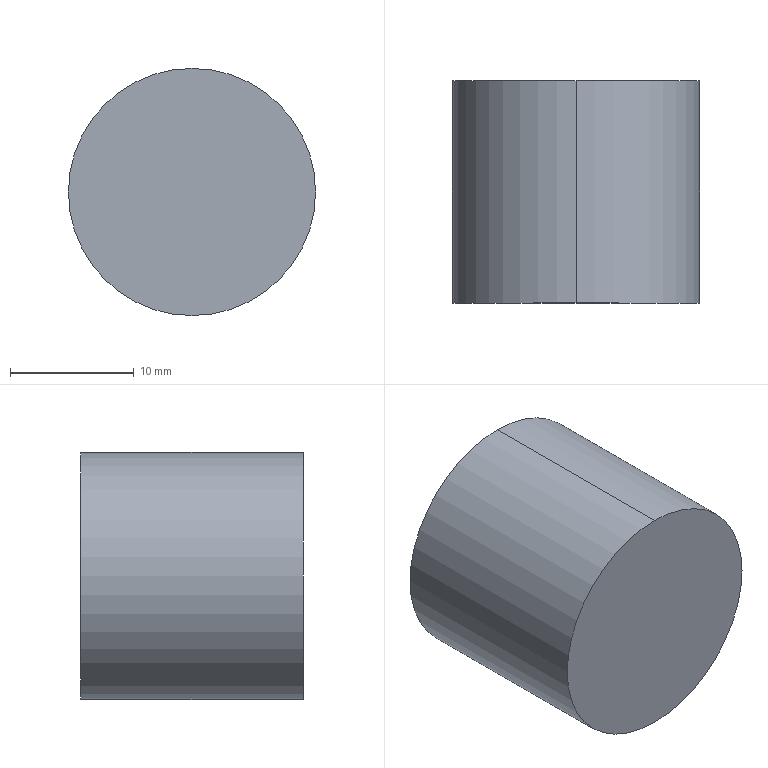Part | STEP file | OP10-158_seal pad (valve guide) | 1 solid | 11 faces | box 20 x 18 x 20 mm | volume 4188 mm3 | cylinder 6 | plane 3 | cone 2 | commonest cylinder face diameters 10 x2 14 x2 20 x2
STEP:
#1=CARTESIAN_POINT('',(0.,0.,0.));
#2=DIRECTION('',(0.,0.,1.));
#3=DIRECTION('',(1.,0.,0.));
#4=AXIS2_PLACEMENT_3D('',#1,#2,#3);
#5=CARTESIAN_POINT('',(0.,7.,5.));
#6=VERTEX_POINT('',#5);
#7=CARTESIAN_POINT('',(0.,11.,5.));
#8=VERTEX_POINT('',#7);
#9=CARTESIAN_POINT('',(0.,18.,5.));
#10=DIRECTION('',(0.,1.,0.));
#11=VECTOR('',#10,1.);
#12=LINE('',#9,#11);
#13=CARTESIAN_POINT('',(0.,18.,0.));
#14=DIRECTION('',(0.,1.,0.));
#15=DIRECTION('',(0.,0.,1.));
#16=AXIS2_PLACEMENT_3D('',#13,#14,#15);
#17=CYLINDRICAL_SURFACE('',#16,5.);
#18=CARTESIAN_POINT('',(6.283,0.));
#19=DIRECTION('',(0.,1.));
#20=VECTOR('',#19,1.);
#21=LINE('',#18,#20);
#22=(GEOMETRIC_REPRESENTATION_CONTEXT(2)PARAMETRIC_REPRESENTATION_CONTEXT()REPRESENTATION_CONTEXT('',''));
#23=DEFINITIONAL_REPRESENTATION('',(#21),#22);
#24=PCURVE('',#17,#23);
#25=CARTESIAN_POINT('',(0.,18.,0.));
#26=DIRECTION('',(0.,1.,0.));
#27=DIRECTION('',(0.,0.,1.));
#28=AXIS2_PLACEMENT_3D('',#25,#26,#27);
#29=CYLINDRICAL_SURFACE('',#28,5.);
#30=CARTESIAN_POINT('',(0.,0.));
#31=DIRECTION('',(0.,1.));
#32=VECTOR('',#31,1.);
#33=LINE('',#30,#32);
#34=(GEOMETRIC_REPRESENTATION_CONTEXT(2)PARAMETRIC_REPRESENTATION_CONTEXT()REPRESENTATION_CONTEXT('',''));
#35=DEFINITIONAL_REPRESENTATION('',(#33),#34);
#36=PCURVE('',#29,#35);
#37=SURFACE_CURVE('',#12,(#24,#36),.PCURVE_S1.);
#38=EDGE_CURVE('',#6,#8,#37,.T.);
#39=ORIENTED_EDGE('',*,*,#38,.T.);
#40=CARTESIAN_POINT('',(0.,11.,-5.));
#41=VERTEX_POINT('',#40);
#42=CARTESIAN_POINT('',(0.,11.,0.));
#43=DIRECTION('',(0.,-1.,0.));
#44=DIRECTION('',(0.,0.,1.));
#45=AXIS2_PLACEMENT_3D('',#42,#43,#44);
#46=CIRCLE('',#45,5.);
#47=CARTESIAN_POINT('',(6.283,-7.));
#48=DIRECTION('',(-1.,0.));
#49=VECTOR('',#48,1.);
#50=LINE('',#47,#49);
#51=(GEOMETRIC_REPRESENTATION_CONTEXT(2)PARAMETRIC_REPRESENTATION_CONTEXT()REPRESENTATION_CONTEXT('',''));
#52=DEFINITIONAL_REPRESENTATION('',(#50),#51);
#53=PCURVE('',#17,#52);
#54=CARTESIAN_POINT('',(0.,11.,0.));
#55=DIRECTION('',(0.,1.,0.));
#56=DIRECTION('',(0.,0.,1.));
#57=AXIS2_PLACEMENT_3D('',#54,#55,#56);
#58=PLANE('',#57);
#59=CARTESIAN_POINT('',(5.,0.));
#60=CARTESIAN_POINT('',(5.,-8.66));
#61=CARTESIAN_POINT('',(-2.5,-4.33));
#62=CARTESIAN_POINT('',(-10.,0.));
#63=CARTESIAN_POINT('',(-2.5,4.33));
#64=CARTESIAN_POINT('',(5.,8.66));
#65=CARTESIAN_POINT('',(5.,0.));
#66=(BOUNDED_CURVE()B_SPLINE_CURVE(2,(#59,#60,#61,#62,#63,#64,#65),.UNSPECIFIED.,.T.,.F.)B_SPLINE_CURVE_WITH_KNOTS((1,2,2,2,2,1),(-2.094,0.,2.094,4.189,6.283,8.378),.UNSPECIFIED.)CURVE()GEOMETRIC_REPRESENTATION_ITEM()RATIONAL_B_SPLINE_CURVE((1.,0.5,1.,0.5,1.,0.5,1.))REPRESENTATION_ITEM(''));
#67=(GEOMETRIC_REPRESENTATION_CONTEXT(2)PARAMETRIC_REPRESENTATION_CONTEXT()REPRESENTATION_CONTEXT('',''));
#68=DEFINITIONAL_REPRESENTATION('',(#66),#67);
#69=PCURVE('',#58,#68);
#70=SURFACE_CURVE('',#46,(#53,#69),.PCURVE_S1.);
#71=EDGE_CURVE('',#8,#41,#70,.T.);
#72=ORIENTED_EDGE('',*,*,#71,.T.);
#73=CARTESIAN_POINT('',(0.,7.,-5.));
#74=VERTEX_POINT('',#73);
#75=CARTESIAN_POINT('',(0.,18.,-5.));
#76=DIRECTION('',(0.,1.,0.));
#77=VECTOR('',#76,1.);
#78=LINE('',#75,#77);
#79=CARTESIAN_POINT('',(3.142,0.));
#80=DIRECTION('',(0.,1.));
#81=VECTOR('',#80,1.);
#82=LINE('',#79,#81);
#83=(GEOMETRIC_REPRESENTATION_CONTEXT(2)PARAMETRIC_REPRESENTATION_CONTEXT()REPRESENTATION_CONTEXT('',''));
#84=DEFINITIONAL_REPRESENTATION('',(#82),#83);
#85=PCURVE('',#17,#84);
#86=CARTESIAN_POINT('',(3.142,0.));
#87=DIRECTION('',(0.,1.));
#88=VECTOR('',#87,1.);
#89=LINE('',#86,#88);
#90=(GEOMETRIC_REPRESENTATION_CONTEXT(2)PARAMETRIC_REPRESENTATION_CONTEXT()REPRESENTATION_CONTEXT('',''));
#91=DEFINITIONAL_REPRESENTATION('',(#89),#90);
#92=PCURVE('',#29,#91);
#93=SURFACE_CURVE('',#78,(#85,#92),.PCURVE_S1.);
#94=EDGE_CURVE('',#74,#41,#93,.T.);
#95=ORIENTED_EDGE('',*,*,#94,.F.);
#96=CARTESIAN_POINT('',(0.,7.,0.));
#97=DIRECTION('',(0.,1.,0.));
#98=DIRECTION('',(0.,0.,1.));
#99=AXIS2_PLACEMENT_3D('',#96,#97,#98);
#100=CIRCLE('',#99,5.);
#101=CARTESIAN_POINT('',(0.,-11.));
#102=DIRECTION('',(1.,0.));
#103=VECTOR('',#102,1.);
#104=LINE('',#101,#103);
#105=(GEOMETRIC_REPRESENTATION_CONTEXT(2)PARAMETRIC_REPRESENTATION_CONTEXT()REPRESENTATION_CONTEXT('',''));
#106=DEFINITIONAL_REPRESENTATION('',(#104),#105);
#107=PCURVE('',#17,#106);
#108=CARTESIAN_POINT('',(0.,7.,0.));
#109=DIRECTION('',(0.,1.,0.));
#110=DIRECTION('',(0.,0.,1.));
#111=AXIS2_PLACEMENT_3D('',#108,#109,#110);
#112=CONICAL_SURFACE('',#111,5.,1.047);
#113=CARTESIAN_POINT('',(0.,0.));
#114=DIRECTION('',(1.,0.));
#115=VECTOR('',#114,1.);
#116=LINE('',#113,#115);
#117=(GEOMETRIC_REPRESENTATION_CONTEXT(2)PARAMETRIC_REPRESENTATION_CONTEXT()REPRESENTATION_CONTEXT('',''));
#118=DEFINITIONAL_REPRESENTATION('',(#116),#117);
#119=PCURVE('',#112,#118);
#120=SURFACE_CURVE('',#100,(#107,#119),.PCURVE_S1.);
#121=EDGE_CURVE('',#74,#6,#120,.T.);
#122=ORIENTED_EDGE('',*,*,#121,.T.);
#123=EDGE_LOOP('',(#39,#72,#95,#122));
#124=FACE_BOUND('',#123,.F.);
#125=ADVANCED_FACE('',(#124),#17,.F.);
#126=ORIENTED_EDGE('',*,*,#121,.F.);
#127=CARTESIAN_POINT('',(0.,4.113,0.));
#128=VERTEX_POINT('',#127);
#129=CARTESIAN_POINT('',(0.,7.,-5.));
#130=DIRECTION('',(0.,0.5,-0.866));
#131=VECTOR('',#130,1.);
#132=LINE('',#129,#131);
#133=CARTESIAN_POINT('',(3.142,0.));
#134=DIRECTION('',(0.,1.));
#135=VECTOR('',#134,1.);
#136=LINE('',#133,#135);
#137=(GEOMETRIC_REPRESENTATION_CONTEXT(2)PARAMETRIC_REPRESENTATION_CONTEXT()REPRESENTATION_CONTEXT('',''));
#138=DEFINITIONAL_REPRESENTATION('',(#136),#137);
#139=PCURVE('',#112,#138);
#140=CARTESIAN_POINT('',(0.,7.,0.));
#141=DIRECTION('',(0.,1.,0.));
#142=DIRECTION('',(0.,0.,1.));
#143=AXIS2_PLACEMENT_3D('',#140,#141,#142);
#144=CONICAL_SURFACE('',#143,5.,1.047);
#145=CARTESIAN_POINT('',(3.142,0.));
#146=DIRECTION('',(0.,1.));
#147=VECTOR('',#146,1.);
#148=LINE('',#145,#147);
#149=(GEOMETRIC_REPRESENTATION_CONTEXT(2)PARAMETRIC_REPRESENTATION_CONTEXT()REPRESENTATION_CONTEXT('',''));
#150=DEFINITIONAL_REPRESENTATION('',(#148),#149);
#151=PCURVE('',#144,#150);
#152=SURFACE_CURVE('',#132,(#139,#151),.PCURVE_S1.);
#153=EDGE_CURVE('',#128,#74,#152,.T.);
#154=ORIENTED_EDGE('',*,*,#153,.F.);
#155=CARTESIAN_POINT('',(0.,7.,5.));
#156=DIRECTION('',(0.,0.5,0.866));
#157=VECTOR('',#156,1.);
#158=LINE('',#155,#157);
#159=CARTESIAN_POINT('',(6.283,0.));
#160=DIRECTION('',(0.,1.));
#161=VECTOR('',#160,1.);
#162=LINE('',#159,#161);
#163=(GEOMETRIC_REPRESENTATION_CONTEXT(2)PARAMETRIC_REPRESENTATION_CONTEXT()REPRESENTATION_CONTEXT('',''));
#164=DEFINITIONAL_REPRESENTATION('',(#162),#163);
#165=PCURVE('',#112,#164);
#166=CARTESIAN_POINT('',(0.,0.));
#167=DIRECTION('',(0.,1.));
#168=VECTOR('',#167,1.);
#169=LINE('',#166,#168);
#170=(GEOMETRIC_REPRESENTATION_CONTEXT(2)PARAMETRIC_REPRESENTATION_CONTEXT()REPRESENTATION_CONTEXT('',''));
#171=DEFINITIONAL_REPRESENTATION('',(#169),#170);
#172=PCURVE('',#144,#171);
#173=SURFACE_CURVE('',#158,(#165,#172),.PCURVE_S1.);
#174=EDGE_CURVE('',#128,#6,#173,.T.);
#175=ORIENTED_EDGE('',*,*,#174,.T.);
#176=EDGE_LOOP('',(#126,#154,#175));
#177=FACE_BOUND('',#176,.F.);
#178=ADVANCED_FACE('',(#177),#112,.F.);
#179=CARTESIAN_POINT('',(0.,11.,7.));
#180=VERTEX_POINT('',#179);
#181=CARTESIAN_POINT('',(0.,18.,7.));
#182=VERTEX_POINT('',#181);
#183=CARTESIAN_POINT('',(0.,11.,7.));
#184=DIRECTION('',(0.,1.,0.));
#185=VECTOR('',#184,1.);
#186=LINE('',#183,#185);
#187=CARTESIAN_POINT('',(0.,11.,0.));
#188=DIRECTION('',(0.,1.,0.));
#189=DIRECTION('',(0.,0.,1.));
#190=AXIS2_PLACEMENT_3D('',#187,#188,#189);
#191=CYLINDRICAL_SURFACE('',#190,7.);
#192=CARTESIAN_POINT('',(6.283,0.));
#193=DIRECTION('',(0.,1.));
#194=VECTOR('',#193,1.);
#195=LINE('',#192,#194);
#196=(GEOMETRIC_REPRESENTATION_CONTEXT(2)PARAMETRIC_REPRESENTATION_CONTEXT()REPRESENTATION_CONTEXT('',''));
#197=DEFINITIONAL_REPRESENTATION('',(#195),#196);
#198=PCURVE('',#191,#197);
#199=CARTESIAN_POINT('',(0.,11.,0.));
#200=DIRECTION('',(0.,1.,0.));
#201=DIRECTION('',(0.,0.,1.));
#202=AXIS2_PLACEMENT_3D('',#199,#200,#201);
#203=CYLINDRICAL_SURFACE('',#202,7.);
#204=CARTESIAN_POINT('',(0.,0.));
#205=DIRECTION('',(0.,1.));
#206=VECTOR('',#205,1.);
#207=LINE('',#204,#206);
#208=(GEOMETRIC_REPRESENTATION_CONTEXT(2)PARAMETRIC_REPRESENTATION_CONTEXT()REPRESENTATION_CONTEXT('',''));
#209=DEFINITIONAL_REPRESENTATION('',(#207),#208);
#210=PCURVE('',#203,#209);
#211=SURFACE_CURVE('',#186,(#198,#210),.PCURVE_S1.);
#212=EDGE_CURVE('',#180,#182,#211,.T.);
#213=ORIENTED_EDGE('',*,*,#212,.T.);
#214=CARTESIAN_POINT('',(0.,18.,-7.));
#215=VERTEX_POINT('',#214);
#216=CARTESIAN_POINT('',(0.,18.,0.));
#217=DIRECTION('',(0.,1.,0.));
#218=DIRECTION('',(0.,0.,1.));
#219=AXIS2_PLACEMENT_3D('',#216,#217,#218);
#220=CIRCLE('',#219,7.);
#221=CARTESIAN_POINT('',(0.,7.));
#222=DIRECTION('',(1.,0.));
#223=VECTOR('',#222,1.);
#224=LINE('',#221,#223);
#225=(GEOMETRIC_REPRESENTATION_CONTEXT(2)PARAMETRIC_REPRESENTATION_CONTEXT()REPRESENTATION_CONTEXT('',''));
#226=DEFINITIONAL_REPRESENTATION('',(#224),#225);
#227=PCURVE('',#191,#226);
#228=CARTESIAN_POINT('',(0.,18.,0.));
#229=DIRECTION('',(0.,1.,0.));
#230=DIRECTION('',(0.,0.,1.));
#231=AXIS2_PLACEMENT_3D('',#228,#229,#230);
#232=PLANE('',#231);
#233=CARTESIAN_POINT('',(0.,0.));
#234=DIRECTION('',(1.,0.));
#235=AXIS2_PLACEMENT_2D('',#233,#234);
#236=CIRCLE('',#235,7.);
#237=(GEOMETRIC_REPRESENTATION_CONTEXT(2)PARAMETRIC_REPRESENTATION_CONTEXT()REPRESENTATION_CONTEXT('',''));
#238=DEFINITIONAL_REPRESENTATION('',(#236),#237);
#239=PCURVE('',#232,#238);
#240=SURFACE_CURVE('',#220,(#227,#239),.PCURVE_S1.);
#241=EDGE_CURVE('',#215,#182,#240,.T.);
#242=ORIENTED_EDGE('',*,*,#241,.F.);
#243=CARTESIAN_POINT('',(0.,11.,-7.));
#244=VERTEX_POINT('',#243);
#245=CARTESIAN_POINT('',(0.,11.,-7.));
#246=DIRECTION('',(0.,1.,0.));
#247=VECTOR('',#246,1.);
#248=LINE('',#245,#247);
#249=CARTESIAN_POINT('',(3.142,0.));
#250=DIRECTION('',(0.,1.));
#251=VECTOR('',#250,1.);
#252=LINE('',#249,#251);
#253=(GEOMETRIC_REPRESENTATION_CONTEXT(2)PARAMETRIC_REPRESENTATION_CONTEXT()REPRESENTATION_CONTEXT('',''));
#254=DEFINITIONAL_REPRESENTATION('',(#252),#253);
#255=PCURVE('',#191,#254);
#256=CARTESIAN_POINT('',(3.142,0.));
#257=DIRECTION('',(0.,1.));
#258=VECTOR('',#257,1.);
#259=LINE('',#256,#258);
#260=(GEOMETRIC_REPRESENTATION_CONTEXT(2)PARAMETRIC_REPRESENTATION_CONTEXT()REPRESENTATION_CONTEXT('',''));
#261=DEFINITIONAL_REPRESENTATION('',(#259),#260);
#262=PCURVE('',#203,#261);
#263=SURFACE_CURVE('',#248,(#255,#262),.PCURVE_S1.);
#264=EDGE_CURVE('',#244,#215,#263,.T.);
#265=ORIENTED_EDGE('',*,*,#264,.F.);
#266=CARTESIAN_POINT('',(0.,11.,0.));
#267=DIRECTION('',(0.,1.,0.));
#268=DIRECTION('',(0.,0.,1.));
#269=AXIS2_PLACEMENT_3D('',#266,#267,#268);
#270=CIRCLE('',#269,7.);
#271=CARTESIAN_POINT('',(0.,0.));
#272=DIRECTION('',(1.,0.));
#273=VECTOR('',#272,1.);
#274=LINE('',#271,#273);
#275=(GEOMETRIC_REPRESENTATION_CONTEXT(2)PARAMETRIC_REPRESENTATION_CONTEXT()REPRESENTATION_CONTEXT('',''));
#276=DEFINITIONAL_REPRESENTATION('',(#274),#275);
#277=PCURVE('',#191,#276);
#278=CARTESIAN_POINT('',(0.,0.));
#279=DIRECTION('',(1.,0.));
#280=AXIS2_PLACEMENT_2D('',#278,#279);
#281=CIRCLE('',#280,7.);
#282=(GEOMETRIC_REPRESENTATION_CONTEXT(2)PARAMETRIC_REPRESENTATION_CONTEXT()REPRESENTATION_CONTEXT('',''));
#283=DEFINITIONAL_REPRESENTATION('',(#281),#282);
#284=PCURVE('',#58,#283);
#285=SURFACE_CURVE('',#270,(#277,#284),.PCURVE_S1.);
#286=EDGE_CURVE('',#244,#180,#285,.T.);
#287=ORIENTED_EDGE('',*,*,#286,.T.);
#288=EDGE_LOOP('',(#213,#242,#265,#287));
#289=FACE_BOUND('',#288,.F.);
#290=ADVANCED_FACE('',(#289),#191,.F.);
#291=CARTESIAN_POINT('',(0.,18.,10.));
#292=VERTEX_POINT('',#291);
#293=CARTESIAN_POINT('',(0.,18.,-10.));
#294=VERTEX_POINT('',#293);
#295=CARTESIAN_POINT('',(0.,18.,0.));
#296=DIRECTION('',(0.,1.,0.));
#297=DIRECTION('',(0.,0.,1.));
#298=AXIS2_PLACEMENT_3D('',#295,#296,#297);
#299=CIRCLE('',#298,10.);
#300=CARTESIAN_POINT('',(0.,18.,0.));
#301=DIRECTION('',(0.,-1.,0.));
#302=DIRECTION('',(0.,0.,-1.));
#303=AXIS2_PLACEMENT_3D('',#300,#301,#302);
#304=CYLINDRICAL_SURFACE('',#303,10.);
#305=CARTESIAN_POINT('',(3.142,0.));
#306=DIRECTION('',(-1.,0.));
#307=VECTOR('',#306,1.);
#308=LINE('',#305,#307);
#309=(GEOMETRIC_REPRESENTATION_CONTEXT(2)PARAMETRIC_REPRESENTATION_CONTEXT()REPRESENTATION_CONTEXT('',''));
#310=DEFINITIONAL_REPRESENTATION('',(#308),#309);
#311=PCURVE('',#304,#310);
#312=CARTESIAN_POINT('',(0.,0.));
#313=DIRECTION('',(1.,0.));
#314=AXIS2_PLACEMENT_2D('',#312,#313);
#315=CIRCLE('',#314,10.);
#316=(GEOMETRIC_REPRESENTATION_CONTEXT(2)PARAMETRIC_REPRESENTATION_CONTEXT()REPRESENTATION_CONTEXT('',''));
#317=DEFINITIONAL_REPRESENTATION('',(#315),#316);
#318=PCURVE('',#232,#317);
#319=SURFACE_CURVE('',#299,(#311,#318),.PCURVE_S1.);
#320=EDGE_CURVE('',#292,#294,#319,.T.);
#321=ORIENTED_EDGE('',*,*,#320,.F.);
#322=CARTESIAN_POINT('',(0.,0.,10.));
#323=VERTEX_POINT('',#322);
#324=CARTESIAN_POINT('',(0.,18.,10.));
#325=DIRECTION('',(0.,-1.,0.));
#326=VECTOR('',#325,1.);
#327=LINE('',#324,#326);
#328=CARTESIAN_POINT('',(3.142,0.));
#329=DIRECTION('',(0.,1.));
#330=VECTOR('',#329,1.);
#331=LINE('',#328,#330);
#332=(GEOMETRIC_REPRESENTATION_CONTEXT(2)PARAMETRIC_REPRESENTATION_CONTEXT()REPRESENTATION_CONTEXT('',''));
#333=DEFINITIONAL_REPRESENTATION('',(#331),#332);
#334=PCURVE('',#304,#333);
#335=CARTESIAN_POINT('',(0.,18.,0.));
#336=DIRECTION('',(0.,-1.,0.));
#337=DIRECTION('',(0.,0.,-1.));
#338=AXIS2_PLACEMENT_3D('',#335,#336,#337);
#339=CYLINDRICAL_SURFACE('',#338,10.);
#340=CARTESIAN_POINT('',(3.142,0.));
#341=DIRECTION('',(0.,1.));
#342=VECTOR('',#341,1.);
#343=LINE('',#340,#342);
#344=(GEOMETRIC_REPRESENTATION_CONTEXT(2)PARAMETRIC_REPRESENTATION_CONTEXT()REPRESENTATION_CONTEXT('',''));
#345=DEFINITIONAL_REPRESENTATION('',(#343),#344);
#346=PCURVE('',#339,#345);
#347=SURFACE_CURVE('',#327,(#334,#346),.PCURVE_S1.);
#348=EDGE_CURVE('',#292,#323,#347,.T.);
#349=ORIENTED_EDGE('',*,*,#348,.T.);
#350=CARTESIAN_POINT('',(0.,0.,-10.));
#351=VERTEX_POINT('',#350);
#352=CARTESIAN_POINT('',(0.,0.,0.));
#353=DIRECTION('',(0.,1.,0.));
#354=DIRECTION('',(0.,0.,1.));
#355=AXIS2_PLACEMENT_3D('',#352,#353,#354);
#356=CIRCLE('',#355,10.);
#357=CARTESIAN_POINT('',(3.142,18.));
#358=DIRECTION('',(-1.,0.));
#359=VECTOR('',#358,1.);
#360=LINE('',#357,#359);
#361=(GEOMETRIC_REPRESENTATION_CONTEXT(2)PARAMETRIC_REPRESENTATION_CONTEXT()REPRESENTATION_CONTEXT('',''));
#362=DEFINITIONAL_REPRESENTATION('',(#360),#361);
#363=PCURVE('',#304,#362);
#364=CARTESIAN_POINT('',(0.,0.,0.));
#365=DIRECTION('',(0.,1.,0.));
#366=DIRECTION('',(0.,0.,1.));
#367=AXIS2_PLACEMENT_3D('',#364,#365,#366);
#368=PLANE('',#367);
#369=CARTESIAN_POINT('',(0.,0.));
#370=DIRECTION('',(1.,0.));
#371=AXIS2_PLACEMENT_2D('',#369,#370);
#372=CIRCLE('',#371,10.);
#373=(GEOMETRIC_REPRESENTATION_CONTEXT(2)PARAMETRIC_REPRESENTATION_CONTEXT()REPRESENTATION_CONTEXT('',''));
#374=DEFINITIONAL_REPRESENTATION('',(#372),#373);
#375=PCURVE('',#368,#374);
#376=SURFACE_CURVE('',#356,(#363,#375),.PCURVE_S1.);
#377=EDGE_CURVE('',#323,#351,#376,.T.);
#378=ORIENTED_EDGE('',*,*,#377,.T.);
#379=CARTESIAN_POINT('',(0.,18.,-10.));
#380=DIRECTION('',(0.,-1.,0.));
#381=VECTOR('',#380,1.);
#382=LINE('',#379,#381);
#383=CARTESIAN_POINT('',(0.,0.));
#384=DIRECTION('',(0.,1.));
#385=VECTOR('',#384,1.);
#386=LINE('',#383,#385);
#387=(GEOMETRIC_REPRESENTATION_CONTEXT(2)PARAMETRIC_REPRESENTATION_CONTEXT()REPRESENTATION_CONTEXT('',''));
#388=DEFINITIONAL_REPRESENTATION('',(#386),#387);
#389=PCURVE('',#304,#388);
#390=CARTESIAN_POINT('',(6.283,0.));
#391=DIRECTION('',(0.,1.));
#392=VECTOR('',#391,1.);
#393=LINE('',#390,#392);
#394=(GEOMETRIC_REPRESENTATION_CONTEXT(2)PARAMETRIC_REPRESENTATION_CONTEXT()REPRESENTATION_CONTEXT('',''));
#395=DEFINITIONAL_REPRESENTATION('',(#393),#394);
#396=PCURVE('',#339,#395);
#397=SURFACE_CURVE('',#382,(#389,#396),.PCURVE_S1.);
#398=EDGE_CURVE('',#294,#351,#397,.T.);
#399=ORIENTED_EDGE('',*,*,#398,.F.);
#400=EDGE_LOOP('',(#321,#349,#378,#399));
#401=FACE_BOUND('',#400,.T.);
#402=ADVANCED_FACE('',(#401),#304,.T.);
#403=ORIENTED_EDGE('',*,*,#348,.F.);
#404=CARTESIAN_POINT('',(0.,18.,0.));
#405=DIRECTION('',(0.,1.,0.));
#406=DIRECTION('',(0.,0.,1.));
#407=AXIS2_PLACEMENT_3D('',#404,#405,#406);
#408=CIRCLE('',#407,10.);
#409=CARTESIAN_POINT('',(9.425,0.));
#410=DIRECTION('',(-1.,0.));
#411=VECTOR('',#410,1.);
#412=LINE('',#409,#411);
#413=(GEOMETRIC_REPRESENTATION_CONTEXT(2)PARAMETRIC_REPRESENTATION_CONTEXT()REPRESENTATION_CONTEXT('',''));
#414=DEFINITIONAL_REPRESENTATION('',(#412),#413);
#415=PCURVE('',#339,#414);
#416=CARTESIAN_POINT('',(0.,0.));
#417=DIRECTION('',(1.,0.));
#418=AXIS2_PLACEMENT_2D('',#416,#417);
#419=CIRCLE('',#418,10.);
#420=(GEOMETRIC_REPRESENTATION_CONTEXT(2)PARAMETRIC_REPRESENTATION_CONTEXT()REPRESENTATION_CONTEXT('',''));
#421=DEFINITIONAL_REPRESENTATION('',(#419),#420);
#422=PCURVE('',#232,#421);
#423=SURFACE_CURVE('',#408,(#415,#422),.PCURVE_S1.);
#424=EDGE_CURVE('',#294,#292,#423,.T.);
#425=ORIENTED_EDGE('',*,*,#424,.F.);
#426=ORIENTED_EDGE('',*,*,#398,.T.);
#427=CARTESIAN_POINT('',(0.,0.,0.));
#428=DIRECTION('',(0.,1.,0.));
#429=DIRECTION('',(0.,0.,1.));
#430=AXIS2_PLACEMENT_3D('',#427,#428,#429);
#431=CIRCLE('',#430,10.);
#432=CARTESIAN_POINT('',(9.425,18.));
#433=DIRECTION('',(-1.,0.));
#434=VECTOR('',#433,1.);
#435=LINE('',#432,#434);
#436=(GEOMETRIC_REPRESENTATION_CONTEXT(2)PARAMETRIC_REPRESENTATION_CONTEXT()REPRESENTATION_CONTEXT('',''));
#437=DEFINITIONAL_REPRESENTATION('',(#435),#436);
#438=PCURVE('',#339,#437);
#439=CARTESIAN_POINT('',(0.,0.));
#440=DIRECTION('',(1.,0.));
#441=AXIS2_PLACEMENT_2D('',#439,#440);
#442=CIRCLE('',#441,10.);
#443=(GEOMETRIC_REPRESENTATION_CONTEXT(2)PARAMETRIC_REPRESENTATION_CONTEXT()REPRESENTATION_CONTEXT('',''));
#444=DEFINITIONAL_REPRESENTATION('',(#442),#443);
#445=PCURVE('',#368,#444);
#446=SURFACE_CURVE('',#431,(#438,#445),.PCURVE_S1.);
#447=EDGE_CURVE('',#351,#323,#446,.T.);
#448=ORIENTED_EDGE('',*,*,#447,.T.);
#449=EDGE_LOOP('',(#403,#425,#426,#448));
#450=FACE_BOUND('',#449,.T.);
#451=ADVANCED_FACE('',(#450),#339,.T.);
#452=CARTESIAN_POINT('',(0.,18.,0.));
#453=DIRECTION('',(0.,1.,0.));
#454=DIRECTION('',(0.,0.,1.));
#455=AXIS2_PLACEMENT_3D('',#452,#453,#454);
#456=CIRCLE('',#455,7.);
#457=CARTESIAN_POINT('',(0.,0.));
#458=DIRECTION('',(1.,0.));
#459=AXIS2_PLACEMENT_2D('',#457,#458);
#460=CIRCLE('',#459,7.);
#461=(GEOMETRIC_REPRESENTATION_CONTEXT(2)PARAMETRIC_REPRESENTATION_CONTEXT()REPRESENTATION_CONTEXT('',''));
#462=DEFINITIONAL_REPRESENTATION('',(#460),#461);
#463=PCURVE('',#232,#462);
#464=CARTESIAN_POINT('',(0.,7.));
#465=DIRECTION('',(1.,0.));
#466=VECTOR('',#465,1.);
#467=LINE('',#464,#466);
#468=(GEOMETRIC_REPRESENTATION_CONTEXT(2)PARAMETRIC_REPRESENTATION_CONTEXT()REPRESENTATION_CONTEXT('',''));
#469=DEFINITIONAL_REPRESENTATION('',(#467),#468);
#470=PCURVE('',#203,#469);
#471=SURFACE_CURVE('',#456,(#463,#470),.PCURVE_S1.);
#472=EDGE_CURVE('',#182,#215,#471,.T.);
#473=ORIENTED_EDGE('',*,*,#472,.F.);
#474=ORIENTED_EDGE('',*,*,#241,.F.);
#475=EDGE_LOOP('',(#473,#474));
#476=FACE_BOUND('',#475,.T.);
#477=ORIENTED_EDGE('',*,*,#424,.T.);
#478=ORIENTED_EDGE('',*,*,#320,.T.);
#479=EDGE_LOOP('',(#477,#478));
#480=FACE_BOUND('',#479,.T.);
#481=ADVANCED_FACE('',(#476,#480),#232,.T.);
#482=ORIENTED_EDGE('',*,*,#447,.F.);
#483=ORIENTED_EDGE('',*,*,#377,.F.);
#484=EDGE_LOOP('',(#482,#483));
#485=FACE_BOUND('',#484,.T.);
#486=ADVANCED_FACE('',(#485),#368,.F.);
#487=CARTESIAN_POINT('',(0.,11.,0.));
#488=DIRECTION('',(0.,1.,0.));
#489=DIRECTION('',(0.,0.,1.));
#490=AXIS2_PLACEMENT_3D('',#487,#488,#489);
#491=CIRCLE('',#490,7.);
#492=CARTESIAN_POINT('',(0.,0.));
#493=DIRECTION('',(1.,0.));
#494=AXIS2_PLACEMENT_2D('',#492,#493);
#495=CIRCLE('',#494,7.);
#496=(GEOMETRIC_REPRESENTATION_CONTEXT(2)PARAMETRIC_REPRESENTATION_CONTEXT()REPRESENTATION_CONTEXT('',''));
#497=DEFINITIONAL_REPRESENTATION('',(#495),#496);
#498=PCURVE('',#58,#497);
#499=CARTESIAN_POINT('',(0.,0.));
#500=DIRECTION('',(1.,0.));
#501=VECTOR('',#500,1.);
#502=LINE('',#499,#501);
#503=(GEOMETRIC_REPRESENTATION_CONTEXT(2)PARAMETRIC_REPRESENTATION_CONTEXT()REPRESENTATION_CONTEXT('',''));
#504=DEFINITIONAL_REPRESENTATION('',(#502),#503);
#505=PCURVE('',#203,#504);
#506=SURFACE_CURVE('',#491,(#498,#505),.PCURVE_S1.);
#507=EDGE_CURVE('',#180,#244,#506,.T.);
#508=ORIENTED_EDGE('',*,*,#507,.T.);
#509=ORIENTED_EDGE('',*,*,#286,.T.);
#510=EDGE_LOOP('',(#508,#509));
#511=FACE_BOUND('',#510,.T.);
#512=ORIENTED_EDGE('',*,*,#71,.T.);
#513=CARTESIAN_POINT('',(0.,11.,0.));
#514=DIRECTION('',(0.,-1.,0.));
#515=DIRECTION('',(0.,0.,1.));
#516=AXIS2_PLACEMENT_3D('',#513,#514,#515);
#517=CIRCLE('',#516,5.);
#518=CARTESIAN_POINT('',(5.,0.));
#519=CARTESIAN_POINT('',(5.,-8.66));
#520=CARTESIAN_POINT('',(-2.5,-4.33));
#521=CARTESIAN_POINT('',(-10.,0.));
#522=CARTESIAN_POINT('',(-2.5,4.33));
#523=CARTESIAN_POINT('',(5.,8.66));
#524=CARTESIAN_POINT('',(5.,0.));
#525=(BOUNDED_CURVE()B_SPLINE_CURVE(2,(#518,#519,#520,#521,#522,#523,#524),.UNSPECIFIED.,.T.,.F.)B_SPLINE_CURVE_WITH_KNOTS((1,2,2,2,2,1),(-2.094,0.,2.094,4.189,6.283,8.378),.UNSPECIFIED.)CURVE()GEOMETRIC_REPRESENTATION_ITEM()RATIONAL_B_SPLINE_CURVE((1.,0.5,1.,0.5,1.,0.5,1.))REPRESENTATION_ITEM(''));
#526=(GEOMETRIC_REPRESENTATION_CONTEXT(2)PARAMETRIC_REPRESENTATION_CONTEXT()REPRESENTATION_CONTEXT('',''));
#527=DEFINITIONAL_REPRESENTATION('',(#525),#526);
#528=PCURVE('',#58,#527);
#529=CARTESIAN_POINT('',(6.283,-7.));
#530=DIRECTION('',(-1.,0.));
#531=VECTOR('',#530,1.);
#532=LINE('',#529,#531);
#533=(GEOMETRIC_REPRESENTATION_CONTEXT(2)PARAMETRIC_REPRESENTATION_CONTEXT()REPRESENTATION_CONTEXT('',''));
#534=DEFINITIONAL_REPRESENTATION('',(#532),#533);
#535=PCURVE('',#29,#534);
#536=SURFACE_CURVE('',#517,(#528,#535),.PCURVE_S1.);
#537=EDGE_CURVE('',#41,#8,#536,.T.);
#538=ORIENTED_EDGE('',*,*,#537,.T.);
#539=EDGE_LOOP('',(#512,#538));
#540=FACE_BOUND('',#539,.T.);
#541=ADVANCED_FACE('',(#511,#540),#58,.T.);
#542=ORIENTED_EDGE('',*,*,#472,.F.);
#543=ORIENTED_EDGE('',*,*,#212,.F.);
#544=ORIENTED_EDGE('',*,*,#507,.T.);
#545=ORIENTED_EDGE('',*,*,#264,.T.);
#546=EDGE_LOOP('',(#542,#543,#544,#545));
#547=FACE_BOUND('',#546,.F.);
#548=ADVANCED_FACE('',(#547),#203,.F.);
#549=CARTESIAN_POINT('',(0.,7.,0.));
#550=DIRECTION('',(0.,1.,0.));
#551=DIRECTION('',(0.,0.,1.));
#552=AXIS2_PLACEMENT_3D('',#549,#550,#551);
#553=CIRCLE('',#552,5.);
#554=CARTESIAN_POINT('',(0.,0.));
#555=DIRECTION('',(1.,0.));
#556=VECTOR('',#555,1.);
#557=LINE('',#554,#556);
#558=(GEOMETRIC_REPRESENTATION_CONTEXT(2)PARAMETRIC_REPRESENTATION_CONTEXT()REPRESENTATION_CONTEXT('',''));
#559=DEFINITIONAL_REPRESENTATION('',(#557),#558);
#560=PCURVE('',#144,#559);
#561=CARTESIAN_POINT('',(0.,-11.));
#562=DIRECTION('',(1.,0.));
#563=VECTOR('',#562,1.);
#564=LINE('',#561,#563);
#565=(GEOMETRIC_REPRESENTATION_CONTEXT(2)PARAMETRIC_REPRESENTATION_CONTEXT()REPRESENTATION_CONTEXT('',''));
#566=DEFINITIONAL_REPRESENTATION('',(#564),#565);
#567=PCURVE('',#29,#566);
#568=SURFACE_CURVE('',#553,(#560,#567),.PCURVE_S1.);
#569=EDGE_CURVE('',#6,#74,#568,.T.);
#570=ORIENTED_EDGE('',*,*,#569,.F.);
#571=ORIENTED_EDGE('',*,*,#174,.F.);
#572=ORIENTED_EDGE('',*,*,#153,.T.);
#573=EDGE_LOOP('',(#570,#571,#572));
#574=FACE_BOUND('',#573,.F.);
#575=ADVANCED_FACE('',(#574),#144,.F.);
#576=ORIENTED_EDGE('',*,*,#537,.T.);
#577=ORIENTED_EDGE('',*,*,#38,.F.);
#578=ORIENTED_EDGE('',*,*,#569,.T.);
#579=ORIENTED_EDGE('',*,*,#94,.T.);
#580=EDGE_LOOP('',(#576,#577,#578,#579));
#581=FACE_BOUND('',#580,.F.);
#582=ADVANCED_FACE('',(#581),#29,.F.);
#583=CLOSED_SHELL('',(#125,#178,#290,#402,#451,#481,#486,#541,#548,#575,#582));
#584=MANIFOLD_SOLID_BREP('',#583);
#585=(LENGTH_UNIT()NAMED_UNIT(*)SI_UNIT(.MILLI.,.METRE.));
#586=UNCERTAINTY_MEASURE_WITH_UNIT(LENGTH_MEASURE(0.0000001),#585,'','');
#587=(NAMED_UNIT(*)PLANE_ANGLE_UNIT()SI_UNIT($,.RADIAN.));
#588=(NAMED_UNIT(*)SI_UNIT($,.STERADIAN.)SOLID_ANGLE_UNIT());
#589=(GEOMETRIC_REPRESENTATION_CONTEXT(3)GLOBAL_UNCERTAINTY_ASSIGNED_CONTEXT((#586))GLOBAL_UNIT_ASSIGNED_CONTEXT((#585,#587,#588))REPRESENTATION_CONTEXT('',''));
#590=ADVANCED_BREP_SHAPE_REPRESENTATION('',(#4,#584),#589);